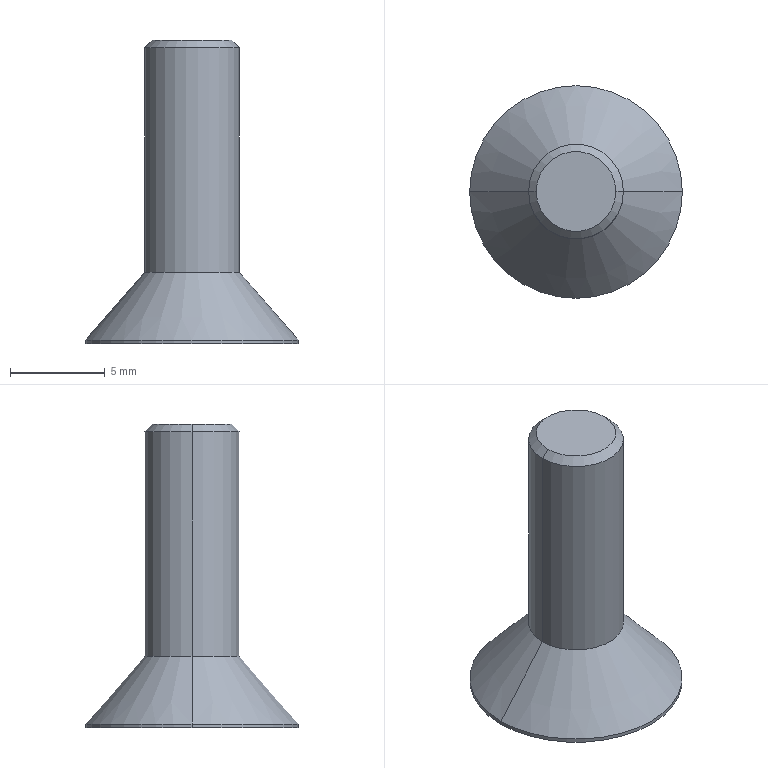Part | Creo | 1 solid | 17 faces | box 11.2 x 11.2 x 16 mm | volume 433.924 mm3 | plane 9 | cylinder 4 | cone 4 | commonest cylinder face diameters 5 x2 11.2 x2
STEP:
#1=CARTESIAN_POINT('',(0.,0.,0.));
#2=DIRECTION('',(0.,0.,1.));
#3=DIRECTION('',(1.,0.,0.));
#4=AXIS2_PLACEMENT_3D('',#1,#2,#3);
#5=CARTESIAN_POINT('',(355.199,-351.929,-27.941));
#6=VERTEX_POINT('',#5);
#7=CARTESIAN_POINT('',(366.399,-351.929,-27.941));
#8=VERTEX_POINT('',#7);
#9=CARTESIAN_POINT('',(360.799,-351.929,-27.941));
#10=DIRECTION('',(0.,0.,-1.));
#11=DIRECTION('',(-1.,0.,0.));
#12=AXIS2_PLACEMENT_3D('',#9,#10,#11);
#13=CIRCLE('',#12,5.6);
#14=EDGE_CURVE('',#6,#8,#13,.T.);
#15=ORIENTED_EDGE('',*,*,#14,.F.);
#16=CARTESIAN_POINT('',(360.799,-351.929,-27.941));
#17=DIRECTION('',(0.,0.,-1.));
#18=DIRECTION('',(1.,0.,0.));
#19=AXIS2_PLACEMENT_3D('',#16,#17,#18);
#20=CIRCLE('',#19,5.6);
#21=EDGE_CURVE('',#8,#6,#20,.T.);
#22=ORIENTED_EDGE('',*,*,#21,.F.);
#23=EDGE_LOOP('',(#15,#22));
#24=FACE_OUTER_BOUND('',#23,.F.);
#25=CARTESIAN_POINT('',(361.549,-350.63,-27.941));
#26=VERTEX_POINT('',#25);
#27=CARTESIAN_POINT('',(360.049,-350.63,-27.941));
#28=VERTEX_POINT('',#27);
#29=CARTESIAN_POINT('',(361.549,-350.63,-27.941));
#30=DIRECTION('',(-1.,0.,0.));
#31=VECTOR('',#30,1.5);
#32=LINE('',#29,#31);
#33=EDGE_CURVE('',#26,#28,#32,.T.);
#34=ORIENTED_EDGE('',*,*,#33,.F.);
#35=CARTESIAN_POINT('',(362.299,-351.929,-27.941));
#36=VERTEX_POINT('',#35);
#37=CARTESIAN_POINT('',(362.299,-351.929,-27.941));
#38=DIRECTION('',(-0.5,0.866,0.));
#39=VECTOR('',#38,1.5);
#40=LINE('',#37,#39);
#41=EDGE_CURVE('',#36,#26,#40,.T.);
#42=ORIENTED_EDGE('',*,*,#41,.F.);
#43=CARTESIAN_POINT('',(361.549,-353.228,-27.941));
#44=VERTEX_POINT('',#43);
#45=CARTESIAN_POINT('',(361.549,-353.228,-27.941));
#46=DIRECTION('',(0.5,0.866,0.));
#47=VECTOR('',#46,1.5);
#48=LINE('',#45,#47);
#49=EDGE_CURVE('',#44,#36,#48,.T.);
#50=ORIENTED_EDGE('',*,*,#49,.F.);
#51=CARTESIAN_POINT('',(360.049,-353.228,-27.941));
#52=VERTEX_POINT('',#51);
#53=CARTESIAN_POINT('',(360.049,-353.228,-27.941));
#54=DIRECTION('',(1.,0.,0.));
#55=VECTOR('',#54,1.5);
#56=LINE('',#53,#55);
#57=EDGE_CURVE('',#52,#44,#56,.T.);
#58=ORIENTED_EDGE('',*,*,#57,.F.);
#59=CARTESIAN_POINT('',(359.299,-351.929,-27.941));
#60=VERTEX_POINT('',#59);
#61=CARTESIAN_POINT('',(359.299,-351.929,-27.941));
#62=DIRECTION('',(0.5,-0.866,0.));
#63=VECTOR('',#62,1.5);
#64=LINE('',#61,#63);
#65=EDGE_CURVE('',#60,#52,#64,.T.);
#66=ORIENTED_EDGE('',*,*,#65,.F.);
#67=CARTESIAN_POINT('',(360.049,-350.63,-27.941));
#68=DIRECTION('',(-0.5,-0.866,0.));
#69=VECTOR('',#68,1.5);
#70=LINE('',#67,#69);
#71=EDGE_CURVE('',#28,#60,#70,.T.);
#72=ORIENTED_EDGE('',*,*,#71,.F.);
#73=EDGE_LOOP('',(#34,#42,#50,#58,#66,#72));
#74=FACE_BOUND('',#73,.F.);
#75=CARTESIAN_POINT('',(360.799,-351.929,-27.941));
#76=DIRECTION('',(0.,0.,-1.));
#77=DIRECTION('',(-1.,0.,0.));
#78=AXIS2_PLACEMENT_3D('',#75,#76,#77);
#79=PLANE('',#78);
#80=ADVANCED_FACE('',(#24,#74),#79,.T.);
#81=ORIENTED_EDGE('',*,*,#33,.T.);
#82=CARTESIAN_POINT('',(360.049,-350.63,-24.941));
#83=VERTEX_POINT('',#82);
#84=CARTESIAN_POINT('',(360.049,-350.63,-27.941));
#85=DIRECTION('',(0.,0.,1.));
#86=VECTOR('',#85,3.);
#87=LINE('',#84,#86);
#88=EDGE_CURVE('',#28,#83,#87,.T.);
#89=ORIENTED_EDGE('',*,*,#88,.T.);
#90=CARTESIAN_POINT('',(361.549,-350.63,-24.941));
#91=VERTEX_POINT('',#90);
#92=CARTESIAN_POINT('',(361.549,-350.63,-24.941));
#93=DIRECTION('',(-1.,0.,0.));
#94=VECTOR('',#93,1.5);
#95=LINE('',#92,#94);
#96=EDGE_CURVE('',#91,#83,#95,.T.);
#97=ORIENTED_EDGE('',*,*,#96,.F.);
#98=CARTESIAN_POINT('',(361.549,-350.63,-27.941));
#99=DIRECTION('',(0.,0.,1.));
#100=VECTOR('',#99,3.);
#101=LINE('',#98,#100);
#102=EDGE_CURVE('',#26,#91,#101,.T.);
#103=ORIENTED_EDGE('',*,*,#102,.F.);
#104=EDGE_LOOP('',(#81,#89,#97,#103));
#105=FACE_OUTER_BOUND('',#104,.F.);
#106=CARTESIAN_POINT('',(360.049,-350.63,-24.941));
#107=DIRECTION('',(0.,1.,0.));
#108=DIRECTION('',(0.,0.,1.));
#109=AXIS2_PLACEMENT_3D('',#106,#107,#108);
#110=PLANE('',#109);
#111=ADVANCED_FACE('',(#105),#110,.F.);
#112=ORIENTED_EDGE('',*,*,#71,.T.);
#113=CARTESIAN_POINT('',(359.299,-351.929,-24.941));
#114=VERTEX_POINT('',#113);
#115=CARTESIAN_POINT('',(359.299,-351.929,-27.941));
#116=DIRECTION('',(0.,0.,1.));
#117=VECTOR('',#116,3.);
#118=LINE('',#115,#117);
#119=EDGE_CURVE('',#60,#114,#118,.T.);
#120=ORIENTED_EDGE('',*,*,#119,.T.);
#121=CARTESIAN_POINT('',(359.299,-351.929,-24.941));
#122=DIRECTION('',(0.5,0.866,0.));
#123=VECTOR('',#122,1.5);
#124=LINE('',#121,#123);
#125=EDGE_CURVE('',#114,#83,#124,.T.);
#126=ORIENTED_EDGE('',*,*,#125,.T.);
#127=ORIENTED_EDGE('',*,*,#88,.F.);
#128=EDGE_LOOP('',(#112,#120,#126,#127));
#129=FACE_OUTER_BOUND('',#128,.F.);
#130=CARTESIAN_POINT('',(359.299,-351.929,-24.941));
#131=DIRECTION('',(-0.866,0.5,0.));
#132=DIRECTION('',(-0.5,-0.866,0.));
#133=AXIS2_PLACEMENT_3D('',#130,#131,#132);
#134=PLANE('',#133);
#135=ADVANCED_FACE('',(#129),#134,.F.);
#136=ORIENTED_EDGE('',*,*,#65,.T.);
#137=CARTESIAN_POINT('',(360.049,-353.228,-24.941));
#138=VERTEX_POINT('',#137);
#139=CARTESIAN_POINT('',(360.049,-353.228,-27.941));
#140=DIRECTION('',(0.,0.,1.));
#141=VECTOR('',#140,3.);
#142=LINE('',#139,#141);
#143=EDGE_CURVE('',#52,#138,#142,.T.);
#144=ORIENTED_EDGE('',*,*,#143,.T.);
#145=CARTESIAN_POINT('',(360.049,-353.228,-24.941));
#146=DIRECTION('',(-0.5,0.866,0.));
#147=VECTOR('',#146,1.5);
#148=LINE('',#145,#147);
#149=EDGE_CURVE('',#138,#114,#148,.T.);
#150=ORIENTED_EDGE('',*,*,#149,.T.);
#151=ORIENTED_EDGE('',*,*,#119,.F.);
#152=EDGE_LOOP('',(#136,#144,#150,#151));
#153=FACE_OUTER_BOUND('',#152,.F.);
#154=CARTESIAN_POINT('',(360.049,-353.228,-24.941));
#155=DIRECTION('',(-0.866,-0.5,0.));
#156=DIRECTION('',(0.5,-0.866,0.));
#157=AXIS2_PLACEMENT_3D('',#154,#155,#156);
#158=PLANE('',#157);
#159=ADVANCED_FACE('',(#153),#158,.F.);
#160=ORIENTED_EDGE('',*,*,#57,.T.);
#161=CARTESIAN_POINT('',(361.549,-353.228,-24.941));
#162=VERTEX_POINT('',#161);
#163=CARTESIAN_POINT('',(361.549,-353.228,-27.941));
#164=DIRECTION('',(0.,0.,1.));
#165=VECTOR('',#164,3.);
#166=LINE('',#163,#165);
#167=EDGE_CURVE('',#44,#162,#166,.T.);
#168=ORIENTED_EDGE('',*,*,#167,.T.);
#169=CARTESIAN_POINT('',(360.049,-353.228,-24.941));
#170=DIRECTION('',(1.,0.,0.));
#171=VECTOR('',#170,1.5);
#172=LINE('',#169,#171);
#173=EDGE_CURVE('',#138,#162,#172,.T.);
#174=ORIENTED_EDGE('',*,*,#173,.F.);
#175=ORIENTED_EDGE('',*,*,#143,.F.);
#176=EDGE_LOOP('',(#160,#168,#174,#175));
#177=FACE_OUTER_BOUND('',#176,.F.);
#178=CARTESIAN_POINT('',(361.549,-353.228,-24.941));
#179=DIRECTION('',(0.,-1.,0.));
#180=DIRECTION('',(0.,0.,-1.));
#181=AXIS2_PLACEMENT_3D('',#178,#179,#180);
#182=PLANE('',#181);
#183=ADVANCED_FACE('',(#177),#182,.F.);
#184=ORIENTED_EDGE('',*,*,#49,.T.);
#185=CARTESIAN_POINT('',(362.299,-351.929,-24.941));
#186=VERTEX_POINT('',#185);
#187=CARTESIAN_POINT('',(362.299,-351.929,-27.941));
#188=DIRECTION('',(0.,0.,1.));
#189=VECTOR('',#188,3.);
#190=LINE('',#187,#189);
#191=EDGE_CURVE('',#36,#186,#190,.T.);
#192=ORIENTED_EDGE('',*,*,#191,.T.);
#193=CARTESIAN_POINT('',(362.299,-351.929,-24.941));
#194=DIRECTION('',(-0.5,-0.866,0.));
#195=VECTOR('',#194,1.5);
#196=LINE('',#193,#195);
#197=EDGE_CURVE('',#186,#162,#196,.T.);
#198=ORIENTED_EDGE('',*,*,#197,.T.);
#199=ORIENTED_EDGE('',*,*,#167,.F.);
#200=EDGE_LOOP('',(#184,#192,#198,#199));
#201=FACE_OUTER_BOUND('',#200,.F.);
#202=CARTESIAN_POINT('',(362.299,-351.929,-24.941));
#203=DIRECTION('',(0.866,-0.5,0.));
#204=DIRECTION('',(0.5,0.866,0.));
#205=AXIS2_PLACEMENT_3D('',#202,#203,#204);
#206=PLANE('',#205);
#207=ADVANCED_FACE('',(#201),#206,.F.);
#208=ORIENTED_EDGE('',*,*,#41,.T.);
#209=ORIENTED_EDGE('',*,*,#102,.T.);
#210=CARTESIAN_POINT('',(361.549,-350.63,-24.941));
#211=DIRECTION('',(0.5,-0.866,0.));
#212=VECTOR('',#211,1.5);
#213=LINE('',#210,#212);
#214=EDGE_CURVE('',#91,#186,#213,.T.);
#215=ORIENTED_EDGE('',*,*,#214,.T.);
#216=ORIENTED_EDGE('',*,*,#191,.F.);
#217=EDGE_LOOP('',(#208,#209,#215,#216));
#218=FACE_OUTER_BOUND('',#217,.F.);
#219=CARTESIAN_POINT('',(361.549,-350.63,-24.941));
#220=DIRECTION('',(0.866,0.5,0.));
#221=DIRECTION('',(-0.5,0.866,0.));
#222=AXIS2_PLACEMENT_3D('',#219,#220,#221);
#223=PLANE('',#222);
#224=ADVANCED_FACE('',(#218),#223,.F.);
#225=ORIENTED_EDGE('',*,*,#96,.T.);
#226=ORIENTED_EDGE('',*,*,#125,.F.);
#227=ORIENTED_EDGE('',*,*,#149,.F.);
#228=ORIENTED_EDGE('',*,*,#173,.T.);
#229=ORIENTED_EDGE('',*,*,#197,.F.);
#230=ORIENTED_EDGE('',*,*,#214,.F.);
#231=EDGE_LOOP('',(#225,#226,#227,#228,#229,#230));
#232=FACE_OUTER_BOUND('',#231,.F.);
#233=CARTESIAN_POINT('',(361.549,-350.63,-24.941));
#234=DIRECTION('',(0.,0.,-1.));
#235=DIRECTION('',(0.,1.,0.));
#236=AXIS2_PLACEMENT_3D('',#233,#234,#235);
#237=PLANE('',#236);
#238=ADVANCED_FACE('',(#232),#237,.T.);
#239=CARTESIAN_POINT('',(366.399,-351.929,-27.741));
#240=VERTEX_POINT('',#239);
#241=CARTESIAN_POINT('',(355.199,-351.929,-27.741));
#242=VERTEX_POINT('',#241);
#243=CARTESIAN_POINT('',(360.799,-351.929,-27.741));
#244=DIRECTION('',(0.,0.,1.));
#245=DIRECTION('',(1.,0.,0.));
#246=AXIS2_PLACEMENT_3D('',#243,#244,#245);
#247=CIRCLE('',#246,5.6);
#248=EDGE_CURVE('',#240,#242,#247,.T.);
#249=ORIENTED_EDGE('',*,*,#248,.T.);
#250=CARTESIAN_POINT('',(355.199,-351.929,-27.741));
#251=DIRECTION('',(0.,0.,-1.));
#252=VECTOR('',#251,0.2);
#253=LINE('',#250,#252);
#254=EDGE_CURVE('',#242,#6,#253,.T.);
#255=ORIENTED_EDGE('',*,*,#254,.T.);
#256=ORIENTED_EDGE('',*,*,#14,.T.);
#257=CARTESIAN_POINT('',(366.399,-351.929,-27.741));
#258=DIRECTION('',(0.,0.,-1.));
#259=VECTOR('',#258,0.2);
#260=LINE('',#257,#259);
#261=EDGE_CURVE('',#240,#8,#260,.T.);
#262=ORIENTED_EDGE('',*,*,#261,.F.);
#263=EDGE_LOOP('',(#249,#255,#256,#262));
#264=FACE_OUTER_BOUND('',#263,.F.);
#265=CARTESIAN_POINT('',(360.799,-351.929,-28.441));
#266=DIRECTION('',(0.,0.,-1.));
#267=DIRECTION('',(-1.,0.,0.));
#268=AXIS2_PLACEMENT_3D('',#265,#266,#267);
#269=CYLINDRICAL_SURFACE('',#268,5.6);
#270=ADVANCED_FACE('',(#264),#269,.T.);
#271=CARTESIAN_POINT('',(358.299,-351.929,-24.175));
#272=VERTEX_POINT('',#271);
#273=CARTESIAN_POINT('',(363.299,-351.929,-24.175));
#274=VERTEX_POINT('',#273);
#275=CARTESIAN_POINT('',(360.799,-351.929,-24.175));
#276=DIRECTION('',(0.,0.,-1.));
#277=DIRECTION('',(-1.,0.,0.));
#278=AXIS2_PLACEMENT_3D('',#275,#276,#277);
#279=CIRCLE('',#278,2.5);
#280=EDGE_CURVE('',#272,#274,#279,.T.);
#281=ORIENTED_EDGE('',*,*,#280,.F.);
#282=CARTESIAN_POINT('',(358.299,-351.929,-24.175));
#283=DIRECTION('',(-0.6561,0.,-0.7547));
#284=VECTOR('',#283,4.725);
#285=LINE('',#282,#284);
#286=EDGE_CURVE('',#272,#242,#285,.T.);
#287=ORIENTED_EDGE('',*,*,#286,.T.);
#288=ORIENTED_EDGE('',*,*,#248,.F.);
#289=CARTESIAN_POINT('',(363.299,-351.929,-24.175));
#290=DIRECTION('',(0.6561,0.,-0.7547));
#291=VECTOR('',#290,4.725);
#292=LINE('',#289,#291);
#293=EDGE_CURVE('',#274,#240,#292,.T.);
#294=ORIENTED_EDGE('',*,*,#293,.F.);
#295=EDGE_LOOP('',(#281,#287,#288,#294));
#296=FACE_OUTER_BOUND('',#295,.F.);
#297=CARTESIAN_POINT('',(360.799,-351.929,-25.958));
#298=DIRECTION('',(0.,0.,-1.));
#299=DIRECTION('',(-1.,0.,0.));
#300=AXIS2_PLACEMENT_3D('',#297,#298,#299);
#301=CONICAL_SURFACE('',#300,4.05,41.);
#302=ADVANCED_FACE('',(#296),#301,.T.);
#303=CARTESIAN_POINT('',(363.299,-351.929,-12.341));
#304=VERTEX_POINT('',#303);
#305=CARTESIAN_POINT('',(358.299,-351.929,-12.341));
#306=VERTEX_POINT('',#305);
#307=CARTESIAN_POINT('',(360.799,-351.929,-12.341));
#308=DIRECTION('',(0.,0.,1.));
#309=DIRECTION('',(1.,0.,0.));
#310=AXIS2_PLACEMENT_3D('',#307,#308,#309);
#311=CIRCLE('',#310,2.5);
#312=EDGE_CURVE('',#304,#306,#311,.T.);
#313=ORIENTED_EDGE('',*,*,#312,.T.);
#314=CARTESIAN_POINT('',(358.299,-351.929,-12.341));
#315=DIRECTION('',(0.,0.,-1.));
#316=VECTOR('',#315,11.834);
#317=LINE('',#314,#316);
#318=EDGE_CURVE('',#306,#272,#317,.T.);
#319=ORIENTED_EDGE('',*,*,#318,.T.);
#320=ORIENTED_EDGE('',*,*,#280,.T.);
#321=CARTESIAN_POINT('',(363.299,-351.929,-12.341));
#322=DIRECTION('',(0.,0.,-1.));
#323=VECTOR('',#322,11.834);
#324=LINE('',#321,#323);
#325=EDGE_CURVE('',#304,#274,#324,.T.);
#326=ORIENTED_EDGE('',*,*,#325,.F.);
#327=EDGE_LOOP('',(#313,#319,#320,#326));
#328=FACE_OUTER_BOUND('',#327,.F.);
#329=CARTESIAN_POINT('',(360.799,-351.929,-28.441));
#330=DIRECTION('',(0.,0.,-1.));
#331=DIRECTION('',(-1.,0.,0.));
#332=AXIS2_PLACEMENT_3D('',#329,#330,#331);
#333=CYLINDRICAL_SURFACE('',#332,2.5);
#334=ADVANCED_FACE('',(#328),#333,.T.);
#335=CARTESIAN_POINT('',(362.899,-351.929,-11.941));
#336=VERTEX_POINT('',#335);
#337=CARTESIAN_POINT('',(358.699,-351.929,-11.941));
#338=VERTEX_POINT('',#337);
#339=CARTESIAN_POINT('',(360.799,-351.929,-11.941));
#340=DIRECTION('',(0.,0.,1.));
#341=DIRECTION('',(1.,0.,0.));
#342=AXIS2_PLACEMENT_3D('',#339,#340,#341);
#343=CIRCLE('',#342,2.1);
#344=EDGE_CURVE('',#336,#338,#343,.T.);
#345=ORIENTED_EDGE('',*,*,#344,.T.);
#346=CARTESIAN_POINT('',(358.699,-351.929,-11.941));
#347=DIRECTION('',(-0.7071,0.,-0.7071));
#348=VECTOR('',#347,0.5657);
#349=LINE('',#346,#348);
#350=EDGE_CURVE('',#338,#306,#349,.T.);
#351=ORIENTED_EDGE('',*,*,#350,.T.);
#352=ORIENTED_EDGE('',*,*,#312,.F.);
#353=CARTESIAN_POINT('',(362.899,-351.929,-11.941));
#354=DIRECTION('',(0.7071,0.,-0.7071));
#355=VECTOR('',#354,0.5657);
#356=LINE('',#353,#355);
#357=EDGE_CURVE('',#336,#304,#356,.T.);
#358=ORIENTED_EDGE('',*,*,#357,.F.);
#359=EDGE_LOOP('',(#345,#351,#352,#358));
#360=FACE_OUTER_BOUND('',#359,.F.);
#361=CARTESIAN_POINT('',(360.799,-351.929,-12.141));
#362=DIRECTION('',(0.,0.,-1.));
#363=DIRECTION('',(-1.,0.,0.));
#364=AXIS2_PLACEMENT_3D('',#361,#362,#363);
#365=CONICAL_SURFACE('',#364,2.3,45.);
#366=ADVANCED_FACE('',(#360),#365,.T.);
#367=ORIENTED_EDGE('',*,*,#344,.F.);
#368=CARTESIAN_POINT('',(360.799,-351.929,-11.941));
#369=DIRECTION('',(0.,0.,1.));
#370=DIRECTION('',(-1.,0.,0.));
#371=AXIS2_PLACEMENT_3D('',#368,#369,#370);
#372=CIRCLE('',#371,2.1);
#373=EDGE_CURVE('',#338,#336,#372,.T.);
#374=ORIENTED_EDGE('',*,*,#373,.F.);
#375=EDGE_LOOP('',(#367,#374));
#376=FACE_OUTER_BOUND('',#375,.F.);
#377=CARTESIAN_POINT('',(358.299,-351.929,-11.941));
#378=DIRECTION('',(0.,0.,1.));
#379=DIRECTION('',(1.,0.,0.));
#380=AXIS2_PLACEMENT_3D('',#377,#378,#379);
#381=PLANE('',#380);
#382=ADVANCED_FACE('',(#376),#381,.T.);
#383=ORIENTED_EDGE('',*,*,#373,.T.);
#384=ORIENTED_EDGE('',*,*,#357,.T.);
#385=CARTESIAN_POINT('',(360.799,-351.929,-12.341));
#386=DIRECTION('',(0.,0.,1.));
#387=DIRECTION('',(-1.,0.,0.));
#388=AXIS2_PLACEMENT_3D('',#385,#386,#387);
#389=CIRCLE('',#388,2.5);
#390=EDGE_CURVE('',#306,#304,#389,.T.);
#391=ORIENTED_EDGE('',*,*,#390,.F.);
#392=ORIENTED_EDGE('',*,*,#350,.F.);
#393=EDGE_LOOP('',(#383,#384,#391,#392));
#394=FACE_OUTER_BOUND('',#393,.F.);
#395=CARTESIAN_POINT('',(360.799,-351.929,-12.141));
#396=DIRECTION('',(0.,0.,-1.));
#397=DIRECTION('',(-1.,0.,0.));
#398=AXIS2_PLACEMENT_3D('',#395,#396,#397);
#399=CONICAL_SURFACE('',#398,2.3,45.);
#400=ADVANCED_FACE('',(#394),#399,.T.);
#401=ORIENTED_EDGE('',*,*,#390,.T.);
#402=ORIENTED_EDGE('',*,*,#325,.T.);
#403=CARTESIAN_POINT('',(360.799,-351.929,-24.175));
#404=DIRECTION('',(0.,0.,-1.));
#405=DIRECTION('',(1.,0.,0.));
#406=AXIS2_PLACEMENT_3D('',#403,#404,#405);
#407=CIRCLE('',#406,2.5);
#408=EDGE_CURVE('',#274,#272,#407,.T.);
#409=ORIENTED_EDGE('',*,*,#408,.T.);
#410=ORIENTED_EDGE('',*,*,#318,.F.);
#411=EDGE_LOOP('',(#401,#402,#409,#410));
#412=FACE_OUTER_BOUND('',#411,.F.);
#413=CARTESIAN_POINT('',(360.799,-351.929,-28.441));
#414=DIRECTION('',(0.,0.,-1.));
#415=DIRECTION('',(-1.,0.,0.));
#416=AXIS2_PLACEMENT_3D('',#413,#414,#415);
#417=CYLINDRICAL_SURFACE('',#416,2.5);
#418=ADVANCED_FACE('',(#412),#417,.T.);
#419=ORIENTED_EDGE('',*,*,#408,.F.);
#420=ORIENTED_EDGE('',*,*,#293,.T.);
#421=CARTESIAN_POINT('',(360.799,-351.929,-27.741));
#422=DIRECTION('',(0.,0.,1.));
#423=DIRECTION('',(-1.,0.,0.));
#424=AXIS2_PLACEMENT_3D('',#421,#422,#423);
#425=CIRCLE('',#424,5.6);
#426=EDGE_CURVE('',#242,#240,#425,.T.);
#427=ORIENTED_EDGE('',*,*,#426,.F.);
#428=ORIENTED_EDGE('',*,*,#286,.F.);
#429=EDGE_LOOP('',(#419,#420,#427,#428));
#430=FACE_OUTER_BOUND('',#429,.F.);
#431=CARTESIAN_POINT('',(360.799,-351.929,-25.958));
#432=DIRECTION('',(0.,0.,-1.));
#433=DIRECTION('',(-1.,0.,0.));
#434=AXIS2_PLACEMENT_3D('',#431,#432,#433);
#435=CONICAL_SURFACE('',#434,4.05,41.);
#436=ADVANCED_FACE('',(#430),#435,.T.);
#437=ORIENTED_EDGE('',*,*,#426,.T.);
#438=ORIENTED_EDGE('',*,*,#261,.T.);
#439=ORIENTED_EDGE('',*,*,#21,.T.);
#440=ORIENTED_EDGE('',*,*,#254,.F.);
#441=EDGE_LOOP('',(#437,#438,#439,#440));
#442=FACE_OUTER_BOUND('',#441,.F.);
#443=CARTESIAN_POINT('',(360.799,-351.929,-28.441));
#444=DIRECTION('',(0.,0.,-1.));
#445=DIRECTION('',(-1.,0.,0.));
#446=AXIS2_PLACEMENT_3D('',#443,#444,#445);
#447=CYLINDRICAL_SURFACE('',#446,5.6);
#448=ADVANCED_FACE('',(#442),#447,.T.);
#449=CLOSED_SHELL('',(#80,#111,#135,#159,#183,#207,#224,#238,#270,#302,#334,#366,#382,#400,#418,#436,#448));
#450=MANIFOLD_SOLID_BREP('',#449);
#451=(LENGTH_UNIT()NAMED_UNIT(*)SI_UNIT(.MILLI.,.METRE.));
#452=UNCERTAINTY_MEASURE_WITH_UNIT(LENGTH_MEASURE(0.002252),#451,'','');
#453=(NAMED_UNIT(*)PLANE_ANGLE_UNIT()SI_UNIT($,.RADIAN.));
#454=PLANE_ANGLE_MEASURE_WITH_UNIT(PLANE_ANGLE_MEASURE(0.01745),#453);
#455=(CONVERSION_BASED_UNIT('DEGREE',#454)NAMED_UNIT(*)PLANE_ANGLE_UNIT());
#456=(NAMED_UNIT(*)SI_UNIT($,.STERADIAN.)SOLID_ANGLE_UNIT());
#457=(GEOMETRIC_REPRESENTATION_CONTEXT(3)GLOBAL_UNCERTAINTY_ASSIGNED_CONTEXT((#452))GLOBAL_UNIT_ASSIGNED_CONTEXT((#451,#455,#456))REPRESENTATION_CONTEXT('',''));
#458=ADVANCED_BREP_SHAPE_REPRESENTATION('',(#4,#450),#457);